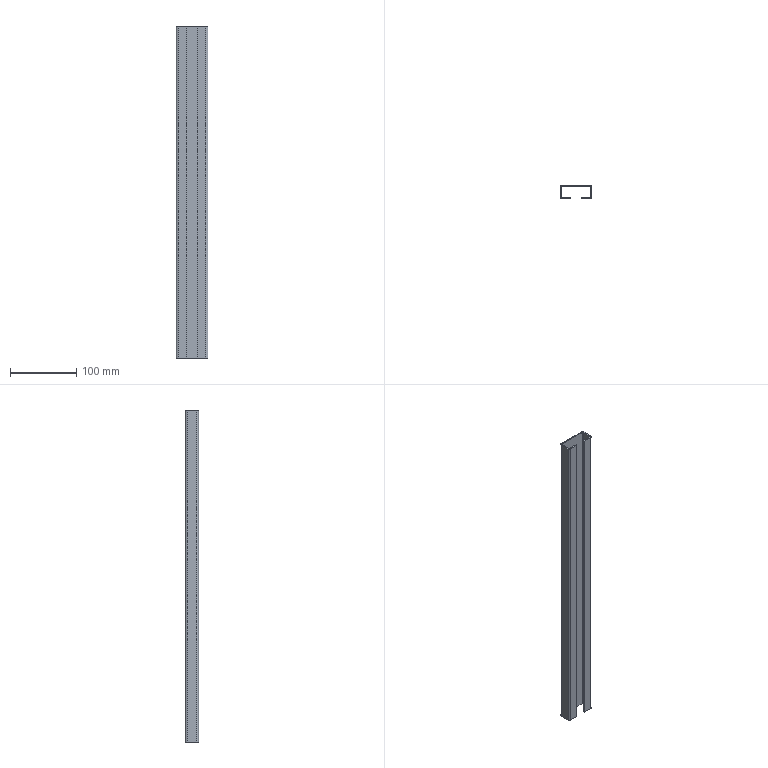Part | SolidWorks | features FlatPattern 1, SMBaseFlange 1, SheetMetal 1 | 1 solid | 38 faces | box 48 x 20 x 500 mm | volume 108566 mm3 | plane 30 | cylinder 8 | commonest cylinder face diameters 2 x4 6 x4
STEP:
#1=CARTESIAN_POINT('',(-24.,-17.,250.));
#2=VERTEX_POINT('',#1);
#3=CARTESIAN_POINT('',(-22.,-17.,250.));
#4=VERTEX_POINT('',#3);
#5=CARTESIAN_POINT('',(-24.,-17.,250.));
#6=DIRECTION('',(1.,0.,0.));
#7=VECTOR('',#6,1000.);
#8=LINE('',#5,#7);
#9=EDGE_CURVE('',#2,#4,#8,.T.);
#10=ORIENTED_EDGE('',*,*,#9,.F.);
#11=CARTESIAN_POINT('',(-21.,-20.,250.));
#12=VERTEX_POINT('',#11);
#13=CARTESIAN_POINT('',(-21.,-17.,250.));
#14=DIRECTION('',(0.,0.,-1.));
#15=DIRECTION('',(1.,0.,0.));
#16=AXIS2_PLACEMENT_3D('',#13,#14,#15);
#17=CIRCLE('',#16,3.);
#18=EDGE_CURVE('',#12,#2,#17,.T.);
#19=ORIENTED_EDGE('',*,*,#18,.F.);
#20=CARTESIAN_POINT('',(-21.,-18.,250.));
#21=VERTEX_POINT('',#20);
#22=CARTESIAN_POINT('',(-21.,-18.,250.));
#23=DIRECTION('',(0.,-1.,0.));
#24=VECTOR('',#23,1000.);
#25=LINE('',#22,#24);
#26=EDGE_CURVE('',#21,#12,#25,.T.);
#27=ORIENTED_EDGE('',*,*,#26,.F.);
#28=CARTESIAN_POINT('',(-21.,-17.,250.));
#29=DIRECTION('',(0.,0.,-1.));
#30=DIRECTION('',(1.,0.,0.));
#31=AXIS2_PLACEMENT_3D('',#28,#29,#30);
#32=CIRCLE('',#31,1.);
#33=EDGE_CURVE('',#21,#4,#32,.T.);
#34=ORIENTED_EDGE('',*,*,#33,.T.);
#35=EDGE_LOOP('',(#10,#19,#27,#34));
#36=FACE_OUTER_BOUND('',#35,.T.);
#37=CARTESIAN_POINT('',(-24.,-17.,250.));
#38=DIRECTION('',(0.,0.,1.));
#39=DIRECTION('',(1.,0.,0.));
#40=AXIS2_PLACEMENT_3D('',#37,#38,#39);
#41=PLANE('',#40);
#42=ADVANCED_FACE('',(#36),#41,.T.);
#43=CARTESIAN_POINT('',(-24.,-3.,250.));
#44=VERTEX_POINT('',#43);
#45=CARTESIAN_POINT('',(-24.,-20.,250.));
#46=DIRECTION('',(0.,1.,0.));
#47=VECTOR('',#46,1000.);
#48=LINE('',#45,#47);
#49=EDGE_CURVE('',#2,#44,#48,.T.);
#50=ORIENTED_EDGE('',*,*,#49,.F.);
#51=ORIENTED_EDGE('',*,*,#9,.T.);
#52=CARTESIAN_POINT('',(-22.,-3.,250.));
#53=VERTEX_POINT('',#52);
#54=CARTESIAN_POINT('',(-22.,-20.,250.));
#55=DIRECTION('',(0.,1.,0.));
#56=VECTOR('',#55,1000.);
#57=LINE('',#54,#56);
#58=EDGE_CURVE('',#4,#53,#57,.T.);
#59=ORIENTED_EDGE('',*,*,#58,.T.);
#60=CARTESIAN_POINT('',(-22.,-3.,250.));
#61=DIRECTION('',(-1.,0.,0.));
#62=VECTOR('',#61,1000.);
#63=LINE('',#60,#62);
#64=EDGE_CURVE('',#53,#44,#63,.T.);
#65=ORIENTED_EDGE('',*,*,#64,.T.);
#66=EDGE_LOOP('',(#50,#51,#59,#65));
#67=FACE_OUTER_BOUND('',#66,.T.);
#68=CARTESIAN_POINT('',(-21.,-18.,250.));
#69=DIRECTION('',(0.,0.,1.));
#70=DIRECTION('',(1.,0.,0.));
#71=AXIS2_PLACEMENT_3D('',#68,#69,#70);
#72=PLANE('',#71);
#73=ADVANCED_FACE('',(#67),#72,.T.);
#74=CARTESIAN_POINT('',(-21.,-20.,-250.));
#75=VERTEX_POINT('',#74);
#76=CARTESIAN_POINT('',(-21.,-18.,-250.));
#77=VERTEX_POINT('',#76);
#78=CARTESIAN_POINT('',(-21.,-20.,-250.));
#79=DIRECTION('',(0.,1.,0.));
#80=VECTOR('',#79,1000.);
#81=LINE('',#78,#80);
#82=EDGE_CURVE('',#75,#77,#81,.T.);
#83=ORIENTED_EDGE('',*,*,#82,.F.);
#84=CARTESIAN_POINT('',(-24.,-17.,-250.));
#85=VERTEX_POINT('',#84);
#86=CARTESIAN_POINT('',(-21.,-17.,-250.));
#87=DIRECTION('',(0.,0.,-1.));
#88=DIRECTION('',(1.,0.,0.));
#89=AXIS2_PLACEMENT_3D('',#86,#87,#88);
#90=CIRCLE('',#89,3.);
#91=EDGE_CURVE('',#75,#85,#90,.T.);
#92=ORIENTED_EDGE('',*,*,#91,.T.);
#93=CARTESIAN_POINT('',(-22.,-17.,-250.));
#94=VERTEX_POINT('',#93);
#95=CARTESIAN_POINT('',(-22.,-17.,-250.));
#96=DIRECTION('',(-1.,0.,0.));
#97=VECTOR('',#96,1000.);
#98=LINE('',#95,#97);
#99=EDGE_CURVE('',#94,#85,#98,.T.);
#100=ORIENTED_EDGE('',*,*,#99,.F.);
#101=CARTESIAN_POINT('',(-21.,-17.,-250.));
#102=DIRECTION('',(0.,0.,-1.));
#103=DIRECTION('',(1.,0.,0.));
#104=AXIS2_PLACEMENT_3D('',#101,#102,#103);
#105=CIRCLE('',#104,1.);
#106=EDGE_CURVE('',#77,#94,#105,.T.);
#107=ORIENTED_EDGE('',*,*,#106,.F.);
#108=EDGE_LOOP('',(#83,#92,#100,#107));
#109=FACE_OUTER_BOUND('',#108,.T.);
#110=CARTESIAN_POINT('',(-21.,-20.,-250.));
#111=DIRECTION('',(0.,0.,-1.));
#112=DIRECTION('',(-1.,0.,0.));
#113=AXIS2_PLACEMENT_3D('',#110,#111,#112);
#114=PLANE('',#113);
#115=ADVANCED_FACE('',(#109),#114,.T.);
#116=CARTESIAN_POINT('',(-8.,-20.,-250.));
#117=VERTEX_POINT('',#116);
#118=CARTESIAN_POINT('',(-8.,-20.,-250.));
#119=DIRECTION('',(-1.,0.,0.));
#120=VECTOR('',#119,1000.);
#121=LINE('',#118,#120);
#122=EDGE_CURVE('',#117,#75,#121,.T.);
#123=ORIENTED_EDGE('',*,*,#122,.T.);
#124=ORIENTED_EDGE('',*,*,#82,.T.);
#125=CARTESIAN_POINT('',(-8.,-18.,-250.));
#126=VERTEX_POINT('',#125);
#127=CARTESIAN_POINT('',(-8.,-18.,-250.));
#128=DIRECTION('',(-1.,0.,0.));
#129=VECTOR('',#128,1000.);
#130=LINE('',#127,#129);
#131=EDGE_CURVE('',#126,#77,#130,.T.);
#132=ORIENTED_EDGE('',*,*,#131,.F.);
#133=CARTESIAN_POINT('',(-8.,-18.,-250.));
#134=DIRECTION('',(0.,-1.,0.));
#135=VECTOR('',#134,1000.);
#136=LINE('',#133,#135);
#137=EDGE_CURVE('',#126,#117,#136,.T.);
#138=ORIENTED_EDGE('',*,*,#137,.T.);
#139=EDGE_LOOP('',(#123,#124,#132,#138));
#140=FACE_OUTER_BOUND('',#139,.T.);
#141=CARTESIAN_POINT('',(-22.,-17.,-250.));
#142=DIRECTION('',(0.,0.,-1.));
#143=DIRECTION('',(-1.,0.,0.));
#144=AXIS2_PLACEMENT_3D('',#141,#142,#143);
#145=PLANE('',#144);
#146=ADVANCED_FACE('',(#140),#145,.T.);
#147=CARTESIAN_POINT('',(-21.,0.,250.));
#148=VERTEX_POINT('',#147);
#149=CARTESIAN_POINT('',(-21.,-2.,250.));
#150=VERTEX_POINT('',#149);
#151=CARTESIAN_POINT('',(-21.,0.,250.));
#152=DIRECTION('',(0.,-1.,0.));
#153=VECTOR('',#152,1000.);
#154=LINE('',#151,#153);
#155=EDGE_CURVE('',#148,#150,#154,.T.);
#156=ORIENTED_EDGE('',*,*,#155,.F.);
#157=CARTESIAN_POINT('',(-21.,-3.,250.));
#158=DIRECTION('',(0.,0.,-1.));
#159=DIRECTION('',(1.,0.,0.));
#160=AXIS2_PLACEMENT_3D('',#157,#158,#159);
#161=CIRCLE('',#160,3.);
#162=EDGE_CURVE('',#44,#148,#161,.T.);
#163=ORIENTED_EDGE('',*,*,#162,.F.);
#164=ORIENTED_EDGE('',*,*,#64,.F.);
#165=CARTESIAN_POINT('',(-21.,-3.,250.));
#166=DIRECTION('',(0.,0.,-1.));
#167=DIRECTION('',(1.,0.,0.));
#168=AXIS2_PLACEMENT_3D('',#165,#166,#167);
#169=CIRCLE('',#168,1.);
#170=EDGE_CURVE('',#53,#150,#169,.T.);
#171=ORIENTED_EDGE('',*,*,#170,.T.);
#172=EDGE_LOOP('',(#156,#163,#164,#171));
#173=FACE_OUTER_BOUND('',#172,.T.);
#174=CARTESIAN_POINT('',(-21.,0.,250.));
#175=DIRECTION('',(0.,0.,1.));
#176=DIRECTION('',(1.,0.,0.));
#177=AXIS2_PLACEMENT_3D('',#174,#175,#176);
#178=PLANE('',#177);
#179=ADVANCED_FACE('',(#173),#178,.T.);
#180=CARTESIAN_POINT('',(21.,0.,250.));
#181=VERTEX_POINT('',#180);
#182=CARTESIAN_POINT('',(-24.,0.,250.));
#183=DIRECTION('',(1.,0.,0.));
#184=VECTOR('',#183,1000.);
#185=LINE('',#182,#184);
#186=EDGE_CURVE('',#148,#181,#185,.T.);
#187=ORIENTED_EDGE('',*,*,#186,.F.);
#188=ORIENTED_EDGE('',*,*,#155,.T.);
#189=CARTESIAN_POINT('',(21.,-2.,250.));
#190=VERTEX_POINT('',#189);
#191=CARTESIAN_POINT('',(-24.,-2.,250.));
#192=DIRECTION('',(1.,0.,0.));
#193=VECTOR('',#192,1000.);
#194=LINE('',#191,#193);
#195=EDGE_CURVE('',#150,#190,#194,.T.);
#196=ORIENTED_EDGE('',*,*,#195,.T.);
#197=CARTESIAN_POINT('',(21.,-2.,250.));
#198=DIRECTION('',(0.,1.,0.));
#199=VECTOR('',#198,1000.);
#200=LINE('',#197,#199);
#201=EDGE_CURVE('',#190,#181,#200,.T.);
#202=ORIENTED_EDGE('',*,*,#201,.T.);
#203=EDGE_LOOP('',(#187,#188,#196,#202));
#204=FACE_OUTER_BOUND('',#203,.T.);
#205=CARTESIAN_POINT('',(-22.,-3.,250.));
#206=DIRECTION('',(0.,0.,1.));
#207=DIRECTION('',(1.,0.,0.));
#208=AXIS2_PLACEMENT_3D('',#205,#206,#207);
#209=PLANE('',#208);
#210=ADVANCED_FACE('',(#204),#209,.T.);
#211=CARTESIAN_POINT('',(-24.,-3.,-250.));
#212=VERTEX_POINT('',#211);
#213=CARTESIAN_POINT('',(-22.,-3.,-250.));
#214=VERTEX_POINT('',#213);
#215=CARTESIAN_POINT('',(-24.,-3.,-250.));
#216=DIRECTION('',(1.,0.,0.));
#217=VECTOR('',#216,1000.);
#218=LINE('',#215,#217);
#219=EDGE_CURVE('',#212,#214,#218,.T.);
#220=ORIENTED_EDGE('',*,*,#219,.F.);
#221=CARTESIAN_POINT('',(-21.,0.,-250.));
#222=VERTEX_POINT('',#221);
#223=CARTESIAN_POINT('',(-21.,-3.,-250.));
#224=DIRECTION('',(0.,0.,-1.));
#225=DIRECTION('',(1.,0.,0.));
#226=AXIS2_PLACEMENT_3D('',#223,#224,#225);
#227=CIRCLE('',#226,3.);
#228=EDGE_CURVE('',#212,#222,#227,.T.);
#229=ORIENTED_EDGE('',*,*,#228,.T.);
#230=CARTESIAN_POINT('',(-21.,-2.,-250.));
#231=VERTEX_POINT('',#230);
#232=CARTESIAN_POINT('',(-21.,-2.,-250.));
#233=DIRECTION('',(0.,1.,0.));
#234=VECTOR('',#233,1000.);
#235=LINE('',#232,#234);
#236=EDGE_CURVE('',#231,#222,#235,.T.);
#237=ORIENTED_EDGE('',*,*,#236,.F.);
#238=CARTESIAN_POINT('',(-21.,-3.,-250.));
#239=DIRECTION('',(0.,0.,-1.));
#240=DIRECTION('',(1.,0.,0.));
#241=AXIS2_PLACEMENT_3D('',#238,#239,#240);
#242=CIRCLE('',#241,1.);
#243=EDGE_CURVE('',#214,#231,#242,.T.);
#244=ORIENTED_EDGE('',*,*,#243,.F.);
#245=EDGE_LOOP('',(#220,#229,#237,#244));
#246=FACE_OUTER_BOUND('',#245,.T.);
#247=CARTESIAN_POINT('',(-24.,-3.,-250.));
#248=DIRECTION('',(0.,0.,-1.));
#249=DIRECTION('',(-1.,0.,0.));
#250=AXIS2_PLACEMENT_3D('',#247,#248,#249);
#251=PLANE('',#250);
#252=ADVANCED_FACE('',(#246),#251,.T.);
#253=CARTESIAN_POINT('',(-24.,-20.,-250.));
#254=DIRECTION('',(0.,1.,0.));
#255=VECTOR('',#254,1000.);
#256=LINE('',#253,#255);
#257=EDGE_CURVE('',#85,#212,#256,.T.);
#258=ORIENTED_EDGE('',*,*,#257,.T.);
#259=ORIENTED_EDGE('',*,*,#219,.T.);
#260=CARTESIAN_POINT('',(-22.,-20.,-250.));
#261=DIRECTION('',(0.,1.,0.));
#262=VECTOR('',#261,1000.);
#263=LINE('',#260,#262);
#264=EDGE_CURVE('',#94,#214,#263,.T.);
#265=ORIENTED_EDGE('',*,*,#264,.F.);
#266=ORIENTED_EDGE('',*,*,#99,.T.);
#267=EDGE_LOOP('',(#258,#259,#265,#266));
#268=FACE_OUTER_BOUND('',#267,.T.);
#269=CARTESIAN_POINT('',(-21.,-2.,-250.));
#270=DIRECTION('',(0.,0.,-1.));
#271=DIRECTION('',(-1.,0.,0.));
#272=AXIS2_PLACEMENT_3D('',#269,#270,#271);
#273=PLANE('',#272);
#274=ADVANCED_FACE('',(#268),#273,.T.);
#275=CARTESIAN_POINT('',(24.,-3.,250.));
#276=VERTEX_POINT('',#275);
#277=CARTESIAN_POINT('',(22.,-3.,250.));
#278=VERTEX_POINT('',#277);
#279=CARTESIAN_POINT('',(24.,-3.,250.));
#280=DIRECTION('',(-1.,0.,0.));
#281=VECTOR('',#280,1000.);
#282=LINE('',#279,#281);
#283=EDGE_CURVE('',#276,#278,#282,.T.);
#284=ORIENTED_EDGE('',*,*,#283,.F.);
#285=CARTESIAN_POINT('',(21.,-3.,250.));
#286=DIRECTION('',(0.,0.,-1.));
#287=DIRECTION('',(1.,0.,0.));
#288=AXIS2_PLACEMENT_3D('',#285,#286,#287);
#289=CIRCLE('',#288,3.);
#290=EDGE_CURVE('',#181,#276,#289,.T.);
#291=ORIENTED_EDGE('',*,*,#290,.F.);
#292=ORIENTED_EDGE('',*,*,#201,.F.);
#293=CARTESIAN_POINT('',(21.,-3.,250.));
#294=DIRECTION('',(0.,0.,-1.));
#295=DIRECTION('',(1.,0.,0.));
#296=AXIS2_PLACEMENT_3D('',#293,#294,#295);
#297=CIRCLE('',#296,1.);
#298=EDGE_CURVE('',#190,#278,#297,.T.);
#299=ORIENTED_EDGE('',*,*,#298,.T.);
#300=EDGE_LOOP('',(#284,#291,#292,#299));
#301=FACE_OUTER_BOUND('',#300,.T.);
#302=CARTESIAN_POINT('',(24.,-3.,250.));
#303=DIRECTION('',(0.,0.,1.));
#304=DIRECTION('',(1.,0.,0.));
#305=AXIS2_PLACEMENT_3D('',#302,#303,#304);
#306=PLANE('',#305);
#307=ADVANCED_FACE('',(#301),#306,.T.);
#308=CARTESIAN_POINT('',(24.,-17.,250.));
#309=VERTEX_POINT('',#308);
#310=CARTESIAN_POINT('',(24.,0.,250.));
#311=DIRECTION('',(0.,-1.,0.));
#312=VECTOR('',#311,1000.);
#313=LINE('',#310,#312);
#314=EDGE_CURVE('',#276,#309,#313,.T.);
#315=ORIENTED_EDGE('',*,*,#314,.F.);
#316=ORIENTED_EDGE('',*,*,#283,.T.);
#317=CARTESIAN_POINT('',(22.,-17.,250.));
#318=VERTEX_POINT('',#317);
#319=CARTESIAN_POINT('',(22.,0.,250.));
#320=DIRECTION('',(0.,-1.,0.));
#321=VECTOR('',#320,1000.);
#322=LINE('',#319,#321);
#323=EDGE_CURVE('',#278,#318,#322,.T.);
#324=ORIENTED_EDGE('',*,*,#323,.T.);
#325=CARTESIAN_POINT('',(22.,-17.,250.));
#326=DIRECTION('',(1.,0.,0.));
#327=VECTOR('',#326,1000.);
#328=LINE('',#325,#327);
#329=EDGE_CURVE('',#318,#309,#328,.T.);
#330=ORIENTED_EDGE('',*,*,#329,.T.);
#331=EDGE_LOOP('',(#315,#316,#324,#330));
#332=FACE_OUTER_BOUND('',#331,.T.);
#333=CARTESIAN_POINT('',(21.,-2.,250.));
#334=DIRECTION('',(0.,0.,1.));
#335=DIRECTION('',(1.,0.,0.));
#336=AXIS2_PLACEMENT_3D('',#333,#334,#335);
#337=PLANE('',#336);
#338=ADVANCED_FACE('',(#332),#337,.T.);
#339=CARTESIAN_POINT('',(21.,0.,-250.));
#340=VERTEX_POINT('',#339);
#341=CARTESIAN_POINT('',(21.,-2.,-250.));
#342=VERTEX_POINT('',#341);
#343=CARTESIAN_POINT('',(21.,0.,-250.));
#344=DIRECTION('',(0.,-1.,0.));
#345=VECTOR('',#344,1000.);
#346=LINE('',#343,#345);
#347=EDGE_CURVE('',#340,#342,#346,.T.);
#348=ORIENTED_EDGE('',*,*,#347,.F.);
#349=CARTESIAN_POINT('',(24.,-3.,-250.));
#350=VERTEX_POINT('',#349);
#351=CARTESIAN_POINT('',(21.,-3.,-250.));
#352=DIRECTION('',(0.,0.,-1.));
#353=DIRECTION('',(1.,0.,0.));
#354=AXIS2_PLACEMENT_3D('',#351,#352,#353);
#355=CIRCLE('',#354,3.);
#356=EDGE_CURVE('',#340,#350,#355,.T.);
#357=ORIENTED_EDGE('',*,*,#356,.T.);
#358=CARTESIAN_POINT('',(22.,-3.,-250.));
#359=VERTEX_POINT('',#358);
#360=CARTESIAN_POINT('',(22.,-3.,-250.));
#361=DIRECTION('',(1.,0.,0.));
#362=VECTOR('',#361,1000.);
#363=LINE('',#360,#362);
#364=EDGE_CURVE('',#359,#350,#363,.T.);
#365=ORIENTED_EDGE('',*,*,#364,.F.);
#366=CARTESIAN_POINT('',(21.,-3.,-250.));
#367=DIRECTION('',(0.,0.,-1.));
#368=DIRECTION('',(1.,0.,0.));
#369=AXIS2_PLACEMENT_3D('',#366,#367,#368);
#370=CIRCLE('',#369,1.);
#371=EDGE_CURVE('',#342,#359,#370,.T.);
#372=ORIENTED_EDGE('',*,*,#371,.F.);
#373=EDGE_LOOP('',(#348,#357,#365,#372));
#374=FACE_OUTER_BOUND('',#373,.T.);
#375=CARTESIAN_POINT('',(21.,0.,-250.));
#376=DIRECTION('',(0.,0.,-1.));
#377=DIRECTION('',(-1.,0.,0.));
#378=AXIS2_PLACEMENT_3D('',#375,#376,#377);
#379=PLANE('',#378);
#380=ADVANCED_FACE('',(#374),#379,.T.);
#381=CARTESIAN_POINT('',(-24.,0.,-250.));
#382=DIRECTION('',(1.,0.,0.));
#383=VECTOR('',#382,1000.);
#384=LINE('',#381,#383);
#385=EDGE_CURVE('',#222,#340,#384,.T.);
#386=ORIENTED_EDGE('',*,*,#385,.T.);
#387=ORIENTED_EDGE('',*,*,#347,.T.);
#388=CARTESIAN_POINT('',(-24.,-2.,-250.));
#389=DIRECTION('',(1.,0.,0.));
#390=VECTOR('',#389,1000.);
#391=LINE('',#388,#390);
#392=EDGE_CURVE('',#231,#342,#391,.T.);
#393=ORIENTED_EDGE('',*,*,#392,.F.);
#394=ORIENTED_EDGE('',*,*,#236,.T.);
#395=EDGE_LOOP('',(#386,#387,#393,#394));
#396=FACE_OUTER_BOUND('',#395,.T.);
#397=CARTESIAN_POINT('',(22.,-3.,-250.));
#398=DIRECTION('',(0.,0.,-1.));
#399=DIRECTION('',(-1.,0.,0.));
#400=AXIS2_PLACEMENT_3D('',#397,#398,#399);
#401=PLANE('',#400);
#402=ADVANCED_FACE('',(#396),#401,.T.);
#403=CARTESIAN_POINT('',(21.,-20.,250.));
#404=VERTEX_POINT('',#403);
#405=CARTESIAN_POINT('',(21.,-18.,250.));
#406=VERTEX_POINT('',#405);
#407=CARTESIAN_POINT('',(21.,-20.,250.));
#408=DIRECTION('',(0.,1.,0.));
#409=VECTOR('',#408,1000.);
#410=LINE('',#407,#409);
#411=EDGE_CURVE('',#404,#406,#410,.T.);
#412=ORIENTED_EDGE('',*,*,#411,.F.);
#413=CARTESIAN_POINT('',(21.,-17.,250.));
#414=DIRECTION('',(0.,0.,-1.));
#415=DIRECTION('',(1.,0.,0.));
#416=AXIS2_PLACEMENT_3D('',#413,#414,#415);
#417=CIRCLE('',#416,3.);
#418=EDGE_CURVE('',#309,#404,#417,.T.);
#419=ORIENTED_EDGE('',*,*,#418,.F.);
#420=ORIENTED_EDGE('',*,*,#329,.F.);
#421=CARTESIAN_POINT('',(21.,-17.,250.));
#422=DIRECTION('',(0.,0.,-1.));
#423=DIRECTION('',(1.,0.,0.));
#424=AXIS2_PLACEMENT_3D('',#421,#422,#423);
#425=CIRCLE('',#424,1.);
#426=EDGE_CURVE('',#318,#406,#425,.T.);
#427=ORIENTED_EDGE('',*,*,#426,.T.);
#428=EDGE_LOOP('',(#412,#419,#420,#427));
#429=FACE_OUTER_BOUND('',#428,.T.);
#430=CARTESIAN_POINT('',(21.,-20.,250.));
#431=DIRECTION('',(0.,0.,1.));
#432=DIRECTION('',(1.,0.,0.));
#433=AXIS2_PLACEMENT_3D('',#430,#431,#432);
#434=PLANE('',#433);
#435=ADVANCED_FACE('',(#429),#434,.T.);
#436=CARTESIAN_POINT('',(8.,-20.,250.));
#437=VERTEX_POINT('',#436);
#438=CARTESIAN_POINT('',(24.,-20.,250.));
#439=DIRECTION('',(-1.,0.,0.));
#440=VECTOR('',#439,1000.);
#441=LINE('',#438,#440);
#442=EDGE_CURVE('',#404,#437,#441,.T.);
#443=ORIENTED_EDGE('',*,*,#442,.F.);
#444=ORIENTED_EDGE('',*,*,#411,.T.);
#445=CARTESIAN_POINT('',(8.,-18.,250.));
#446=VERTEX_POINT('',#445);
#447=CARTESIAN_POINT('',(24.,-18.,250.));
#448=DIRECTION('',(-1.,0.,0.));
#449=VECTOR('',#448,1000.);
#450=LINE('',#447,#449);
#451=EDGE_CURVE('',#406,#446,#450,.T.);
#452=ORIENTED_EDGE('',*,*,#451,.T.);
#453=CARTESIAN_POINT('',(8.,-20.,250.));
#454=DIRECTION('',(0.,1.,0.));
#455=VECTOR('',#454,1000.);
#456=LINE('',#453,#455);
#457=EDGE_CURVE('',#437,#446,#456,.T.);
#458=ORIENTED_EDGE('',*,*,#457,.F.);
#459=EDGE_LOOP('',(#443,#444,#452,#458));
#460=FACE_OUTER_BOUND('',#459,.T.);
#461=CARTESIAN_POINT('',(22.,-17.,250.));
#462=DIRECTION('',(0.,0.,1.));
#463=DIRECTION('',(1.,0.,0.));
#464=AXIS2_PLACEMENT_3D('',#461,#462,#463);
#465=PLANE('',#464);
#466=ADVANCED_FACE('',(#460),#465,.T.);
#467=CARTESIAN_POINT('',(24.,-17.,-250.));
#468=VERTEX_POINT('',#467);
#469=CARTESIAN_POINT('',(22.,-17.,-250.));
#470=VERTEX_POINT('',#469);
#471=CARTESIAN_POINT('',(24.,-17.,-250.));
#472=DIRECTION('',(-1.,0.,0.));
#473=VECTOR('',#472,1000.);
#474=LINE('',#471,#473);
#475=EDGE_CURVE('',#468,#470,#474,.T.);
#476=ORIENTED_EDGE('',*,*,#475,.F.);
#477=CARTESIAN_POINT('',(21.,-20.,-250.));
#478=VERTEX_POINT('',#477);
#479=CARTESIAN_POINT('',(21.,-17.,-250.));
#480=DIRECTION('',(0.,0.,-1.));
#481=DIRECTION('',(1.,0.,0.));
#482=AXIS2_PLACEMENT_3D('',#479,#480,#481);
#483=CIRCLE('',#482,3.);
#484=EDGE_CURVE('',#468,#478,#483,.T.);
#485=ORIENTED_EDGE('',*,*,#484,.T.);
#486=CARTESIAN_POINT('',(21.,-18.,-250.));
#487=VERTEX_POINT('',#486);
#488=CARTESIAN_POINT('',(21.,-18.,-250.));
#489=DIRECTION('',(0.,-1.,0.));
#490=VECTOR('',#489,1000.);
#491=LINE('',#488,#490);
#492=EDGE_CURVE('',#487,#478,#491,.T.);
#493=ORIENTED_EDGE('',*,*,#492,.F.);
#494=CARTESIAN_POINT('',(21.,-17.,-250.));
#495=DIRECTION('',(0.,0.,-1.));
#496=DIRECTION('',(1.,0.,0.));
#497=AXIS2_PLACEMENT_3D('',#494,#495,#496);
#498=CIRCLE('',#497,1.);
#499=EDGE_CURVE('',#470,#487,#498,.T.);
#500=ORIENTED_EDGE('',*,*,#499,.F.);
#501=EDGE_LOOP('',(#476,#485,#493,#500));
#502=FACE_OUTER_BOUND('',#501,.T.);
#503=CARTESIAN_POINT('',(24.,-17.,-250.));
#504=DIRECTION('',(0.,0.,-1.));
#505=DIRECTION('',(-1.,0.,0.));
#506=AXIS2_PLACEMENT_3D('',#503,#504,#505);
#507=PLANE('',#506);
#508=ADVANCED_FACE('',(#502),#507,.T.);
#509=CARTESIAN_POINT('',(24.,0.,-250.));
#510=DIRECTION('',(0.,-1.,0.));
#511=VECTOR('',#510,1000.);
#512=LINE('',#509,#511);
#513=EDGE_CURVE('',#350,#468,#512,.T.);
#514=ORIENTED_EDGE('',*,*,#513,.T.);
#515=ORIENTED_EDGE('',*,*,#475,.T.);
#516=CARTESIAN_POINT('',(22.,0.,-250.));
#517=DIRECTION('',(0.,-1.,0.));
#518=VECTOR('',#517,1000.);
#519=LINE('',#516,#518);
#520=EDGE_CURVE('',#359,#470,#519,.T.);
#521=ORIENTED_EDGE('',*,*,#520,.F.);
#522=ORIENTED_EDGE('',*,*,#364,.T.);
#523=EDGE_LOOP('',(#514,#515,#521,#522));
#524=FACE_OUTER_BOUND('',#523,.T.);
#525=CARTESIAN_POINT('',(21.,-18.,-250.));
#526=DIRECTION('',(0.,0.,-1.));
#527=DIRECTION('',(-1.,0.,0.));
#528=AXIS2_PLACEMENT_3D('',#525,#526,#527);
#529=PLANE('',#528);
#530=ADVANCED_FACE('',(#524),#529,.T.);
#531=CARTESIAN_POINT('',(8.,-18.,-250.));
#532=VERTEX_POINT('',#531);
#533=CARTESIAN_POINT('',(24.,-18.,-250.));
#534=DIRECTION('',(-1.,0.,0.));
#535=VECTOR('',#534,1000.);
#536=LINE('',#533,#535);
#537=EDGE_CURVE('',#487,#532,#536,.T.);
#538=ORIENTED_EDGE('',*,*,#537,.T.);
#539=CARTESIAN_POINT('',(8.,-18.,250.));
#540=DIRECTION('',(0.,0.,-1.));
#541=VECTOR('',#540,1000.);
#542=LINE('',#539,#541);
#543=EDGE_CURVE('',#446,#532,#542,.T.);
#544=ORIENTED_EDGE('',*,*,#543,.F.);
#545=ORIENTED_EDGE('',*,*,#451,.F.);
#546=CARTESIAN_POINT('',(21.,-18.,250.));
#547=DIRECTION('',(0.,0.,-1.));
#548=VECTOR('',#547,1000.);
#549=LINE('',#546,#548);
#550=EDGE_CURVE('',#406,#487,#549,.T.);
#551=ORIENTED_EDGE('',*,*,#550,.T.);
#552=EDGE_LOOP('',(#538,#544,#545,#551));
#553=FACE_OUTER_BOUND('',#552,.T.);
#554=CARTESIAN_POINT('',(24.,-18.,250.));
#555=DIRECTION('',(0.,-1.,0.));
#556=DIRECTION('',(1.,0.,0.));
#557=AXIS2_PLACEMENT_3D('',#554,#555,#556);
#558=PLANE('',#557);
#559=ADVANCED_FACE('',(#553),#558,.F.);
#560=CARTESIAN_POINT('',(8.,-20.,-250.));
#561=VERTEX_POINT('',#560);
#562=CARTESIAN_POINT('',(8.,-20.,-250.));
#563=DIRECTION('',(0.,1.,0.));
#564=VECTOR('',#563,1000.);
#565=LINE('',#562,#564);
#566=EDGE_CURVE('',#561,#532,#565,.T.);
#567=ORIENTED_EDGE('',*,*,#566,.F.);
#568=CARTESIAN_POINT('',(8.,-20.,250.));
#569=DIRECTION('',(0.,0.,-1.));
#570=VECTOR('',#569,1000.);
#571=LINE('',#568,#570);
#572=EDGE_CURVE('',#437,#561,#571,.T.);
#573=ORIENTED_EDGE('',*,*,#572,.F.);
#574=ORIENTED_EDGE('',*,*,#457,.T.);
#575=ORIENTED_EDGE('',*,*,#543,.T.);
#576=EDGE_LOOP('',(#567,#573,#574,#575));
#577=FACE_OUTER_BOUND('',#576,.T.);
#578=CARTESIAN_POINT('',(8.,-20.,250.));
#579=DIRECTION('',(-1.,0.,0.));
#580=DIRECTION('',(0.,0.,1.));
#581=AXIS2_PLACEMENT_3D('',#578,#579,#580);
#582=PLANE('',#581);
#583=ADVANCED_FACE('',(#577),#582,.T.);
#584=CARTESIAN_POINT('',(24.,-20.,-250.));
#585=DIRECTION('',(-1.,0.,0.));
#586=VECTOR('',#585,1000.);
#587=LINE('',#584,#586);
#588=EDGE_CURVE('',#478,#561,#587,.T.);
#589=ORIENTED_EDGE('',*,*,#588,.F.);
#590=CARTESIAN_POINT('',(21.,-20.,250.));
#591=DIRECTION('',(0.,0.,-1.));
#592=VECTOR('',#591,1000.);
#593=LINE('',#590,#592);
#594=EDGE_CURVE('',#404,#478,#593,.T.);
#595=ORIENTED_EDGE('',*,*,#594,.F.);
#596=ORIENTED_EDGE('',*,*,#442,.T.);
#597=ORIENTED_EDGE('',*,*,#572,.T.);
#598=EDGE_LOOP('',(#589,#595,#596,#597));
#599=FACE_OUTER_BOUND('',#598,.T.);
#600=CARTESIAN_POINT('',(24.,-20.,250.));
#601=DIRECTION('',(0.,-1.,0.));
#602=DIRECTION('',(1.,0.,0.));
#603=AXIS2_PLACEMENT_3D('',#600,#601,#602);
#604=PLANE('',#603);
#605=ADVANCED_FACE('',(#599),#604,.T.);
#606=ORIENTED_EDGE('',*,*,#484,.F.);
#607=CARTESIAN_POINT('',(24.,-17.,250.));
#608=DIRECTION('',(0.,0.,-1.));
#609=VECTOR('',#608,1000.);
#610=LINE('',#607,#609);
#611=EDGE_CURVE('',#309,#468,#610,.T.);
#612=ORIENTED_EDGE('',*,*,#611,.F.);
#613=ORIENTED_EDGE('',*,*,#418,.T.);
#614=ORIENTED_EDGE('',*,*,#594,.T.);
#615=EDGE_LOOP('',(#606,#612,#613,#614));
#616=FACE_OUTER_BOUND('',#615,.T.);
#617=CARTESIAN_POINT('',(21.,-17.,250.));
#618=DIRECTION('',(0.,0.,-1.));
#619=DIRECTION('',(-1.,0.,0.));
#620=AXIS2_PLACEMENT_3D('',#617,#618,#619);
#621=CYLINDRICAL_SURFACE('',#620,3.);
#622=ADVANCED_FACE('',(#616),#621,.T.);
#623=ORIENTED_EDGE('',*,*,#513,.F.);
#624=CARTESIAN_POINT('',(24.,-3.,250.));
#625=DIRECTION('',(0.,0.,-1.));
#626=VECTOR('',#625,1000.);
#627=LINE('',#624,#626);
#628=EDGE_CURVE('',#276,#350,#627,.T.);
#629=ORIENTED_EDGE('',*,*,#628,.F.);
#630=ORIENTED_EDGE('',*,*,#314,.T.);
#631=ORIENTED_EDGE('',*,*,#611,.T.);
#632=EDGE_LOOP('',(#623,#629,#630,#631));
#633=FACE_OUTER_BOUND('',#632,.T.);
#634=CARTESIAN_POINT('',(24.,0.,250.));
#635=DIRECTION('',(1.,0.,0.));
#636=DIRECTION('',(0.,0.,-1.));
#637=AXIS2_PLACEMENT_3D('',#634,#635,#636);
#638=PLANE('',#637);
#639=ADVANCED_FACE('',(#633),#638,.T.);
#640=ORIENTED_EDGE('',*,*,#356,.F.);
#641=CARTESIAN_POINT('',(21.,0.,250.));
#642=DIRECTION('',(0.,0.,-1.));
#643=VECTOR('',#642,1000.);
#644=LINE('',#641,#643);
#645=EDGE_CURVE('',#181,#340,#644,.T.);
#646=ORIENTED_EDGE('',*,*,#645,.F.);
#647=ORIENTED_EDGE('',*,*,#290,.T.);
#648=ORIENTED_EDGE('',*,*,#628,.T.);
#649=EDGE_LOOP('',(#640,#646,#647,#648));
#650=FACE_OUTER_BOUND('',#649,.T.);
#651=CARTESIAN_POINT('',(21.,-3.,250.));
#652=DIRECTION('',(0.,0.,-1.));
#653=DIRECTION('',(-1.,0.,0.));
#654=AXIS2_PLACEMENT_3D('',#651,#652,#653);
#655=CYLINDRICAL_SURFACE('',#654,3.);
#656=ADVANCED_FACE('',(#650),#655,.T.);
#657=ORIENTED_EDGE('',*,*,#385,.F.);
#658=CARTESIAN_POINT('',(-21.,0.,250.));
#659=DIRECTION('',(0.,0.,-1.));
#660=VECTOR('',#659,1000.);
#661=LINE('',#658,#660);
#662=EDGE_CURVE('',#148,#222,#661,.T.);
#663=ORIENTED_EDGE('',*,*,#662,.F.);
#664=ORIENTED_EDGE('',*,*,#186,.T.);
#665=ORIENTED_EDGE('',*,*,#645,.T.);
#666=EDGE_LOOP('',(#657,#663,#664,#665));
#667=FACE_OUTER_BOUND('',#666,.T.);
#668=CARTESIAN_POINT('',(-24.,0.,250.));
#669=DIRECTION('',(0.,1.,0.));
#670=DIRECTION('',(0.,0.,1.));
#671=AXIS2_PLACEMENT_3D('',#668,#669,#670);
#672=PLANE('',#671);
#673=ADVANCED_FACE('',(#667),#672,.T.);
#674=ORIENTED_EDGE('',*,*,#228,.F.);
#675=CARTESIAN_POINT('',(-24.,-3.,250.));
#676=DIRECTION('',(0.,0.,-1.));
#677=VECTOR('',#676,1000.);
#678=LINE('',#675,#677);
#679=EDGE_CURVE('',#44,#212,#678,.T.);
#680=ORIENTED_EDGE('',*,*,#679,.F.);
#681=ORIENTED_EDGE('',*,*,#162,.T.);
#682=ORIENTED_EDGE('',*,*,#662,.T.);
#683=EDGE_LOOP('',(#674,#680,#681,#682));
#684=FACE_OUTER_BOUND('',#683,.T.);
#685=CARTESIAN_POINT('',(-21.,-3.,250.));
#686=DIRECTION('',(0.,0.,-1.));
#687=DIRECTION('',(-1.,0.,0.));
#688=AXIS2_PLACEMENT_3D('',#685,#686,#687);
#689=CYLINDRICAL_SURFACE('',#688,3.);
#690=ADVANCED_FACE('',(#684),#689,.T.);
#691=ORIENTED_EDGE('',*,*,#257,.F.);
#692=CARTESIAN_POINT('',(-24.,-17.,250.));
#693=DIRECTION('',(0.,0.,-1.));
#694=VECTOR('',#693,1000.);
#695=LINE('',#692,#694);
#696=EDGE_CURVE('',#2,#85,#695,.T.);
#697=ORIENTED_EDGE('',*,*,#696,.F.);
#698=ORIENTED_EDGE('',*,*,#49,.T.);
#699=ORIENTED_EDGE('',*,*,#679,.T.);
#700=EDGE_LOOP('',(#691,#697,#698,#699));
#701=FACE_OUTER_BOUND('',#700,.T.);
#702=CARTESIAN_POINT('',(-24.,-20.,250.));
#703=DIRECTION('',(-1.,0.,0.));
#704=DIRECTION('',(0.,0.,1.));
#705=AXIS2_PLACEMENT_3D('',#702,#703,#704);
#706=PLANE('',#705);
#707=ADVANCED_FACE('',(#701),#706,.T.);
#708=ORIENTED_EDGE('',*,*,#91,.F.);
#709=CARTESIAN_POINT('',(-21.,-20.,250.));
#710=DIRECTION('',(0.,0.,-1.));
#711=VECTOR('',#710,1000.);
#712=LINE('',#709,#711);
#713=EDGE_CURVE('',#12,#75,#712,.T.);
#714=ORIENTED_EDGE('',*,*,#713,.F.);
#715=ORIENTED_EDGE('',*,*,#18,.T.);
#716=ORIENTED_EDGE('',*,*,#696,.T.);
#717=EDGE_LOOP('',(#708,#714,#715,#716));
#718=FACE_OUTER_BOUND('',#717,.T.);
#719=CARTESIAN_POINT('',(-21.,-17.,250.));
#720=DIRECTION('',(0.,0.,-1.));
#721=DIRECTION('',(-1.,0.,0.));
#722=AXIS2_PLACEMENT_3D('',#719,#720,#721);
#723=CYLINDRICAL_SURFACE('',#722,3.);
#724=ADVANCED_FACE('',(#718),#723,.T.);
#725=ORIENTED_EDGE('',*,*,#122,.F.);
#726=CARTESIAN_POINT('',(-8.,-20.,250.));
#727=VERTEX_POINT('',#726);
#728=CARTESIAN_POINT('',(-8.,-20.,250.));
#729=DIRECTION('',(0.,0.,-1.));
#730=VECTOR('',#729,1000.);
#731=LINE('',#728,#730);
#732=EDGE_CURVE('',#727,#117,#731,.T.);
#733=ORIENTED_EDGE('',*,*,#732,.F.);
#734=CARTESIAN_POINT('',(-8.,-20.,250.));
#735=DIRECTION('',(-1.,0.,0.));
#736=VECTOR('',#735,1000.);
#737=LINE('',#734,#736);
#738=EDGE_CURVE('',#727,#12,#737,.T.);
#739=ORIENTED_EDGE('',*,*,#738,.T.);
#740=ORIENTED_EDGE('',*,*,#713,.T.);
#741=EDGE_LOOP('',(#725,#733,#739,#740));
#742=FACE_OUTER_BOUND('',#741,.T.);
#743=CARTESIAN_POINT('',(-8.,-20.,250.));
#744=DIRECTION('',(0.,-1.,0.));
#745=DIRECTION('',(1.,0.,0.));
#746=AXIS2_PLACEMENT_3D('',#743,#744,#745);
#747=PLANE('',#746);
#748=ADVANCED_FACE('',(#742),#747,.T.);
#749=ORIENTED_EDGE('',*,*,#137,.F.);
#750=CARTESIAN_POINT('',(-8.,-18.,250.));
#751=VERTEX_POINT('',#750);
#752=CARTESIAN_POINT('',(-8.,-18.,250.));
#753=DIRECTION('',(0.,0.,-1.));
#754=VECTOR('',#753,1000.);
#755=LINE('',#752,#754);
#756=EDGE_CURVE('',#751,#126,#755,.T.);
#757=ORIENTED_EDGE('',*,*,#756,.F.);
#758=CARTESIAN_POINT('',(-8.,-18.,250.));
#759=DIRECTION('',(0.,-1.,0.));
#760=VECTOR('',#759,1000.);
#761=LINE('',#758,#760);
#762=EDGE_CURVE('',#751,#727,#761,.T.);
#763=ORIENTED_EDGE('',*,*,#762,.T.);
#764=ORIENTED_EDGE('',*,*,#732,.T.);
#765=EDGE_LOOP('',(#749,#757,#763,#764));
#766=FACE_OUTER_BOUND('',#765,.T.);
#767=CARTESIAN_POINT('',(-8.,-18.,250.));
#768=DIRECTION('',(1.,0.,0.));
#769=DIRECTION('',(0.,0.,-1.));
#770=AXIS2_PLACEMENT_3D('',#767,#768,#769);
#771=PLANE('',#770);
#772=ADVANCED_FACE('',(#766),#771,.T.);
#773=ORIENTED_EDGE('',*,*,#131,.T.);
#774=CARTESIAN_POINT('',(-21.,-18.,250.));
#775=DIRECTION('',(0.,0.,-1.));
#776=VECTOR('',#775,1000.);
#777=LINE('',#774,#776);
#778=EDGE_CURVE('',#21,#77,#777,.T.);
#779=ORIENTED_EDGE('',*,*,#778,.F.);
#780=CARTESIAN_POINT('',(-8.,-18.,250.));
#781=DIRECTION('',(-1.,0.,0.));
#782=VECTOR('',#781,1000.);
#783=LINE('',#780,#782);
#784=EDGE_CURVE('',#751,#21,#783,.T.);
#785=ORIENTED_EDGE('',*,*,#784,.F.);
#786=ORIENTED_EDGE('',*,*,#756,.T.);
#787=EDGE_LOOP('',(#773,#779,#785,#786));
#788=FACE_OUTER_BOUND('',#787,.T.);
#789=CARTESIAN_POINT('',(-8.,-18.,250.));
#790=DIRECTION('',(0.,-1.,0.));
#791=DIRECTION('',(1.,0.,0.));
#792=AXIS2_PLACEMENT_3D('',#789,#790,#791);
#793=PLANE('',#792);
#794=ADVANCED_FACE('',(#788),#793,.F.);
#795=ORIENTED_EDGE('',*,*,#106,.T.);
#796=CARTESIAN_POINT('',(-22.,-17.,250.));
#797=DIRECTION('',(0.,0.,-1.));
#798=VECTOR('',#797,1000.);
#799=LINE('',#796,#798);
#800=EDGE_CURVE('',#4,#94,#799,.T.);
#801=ORIENTED_EDGE('',*,*,#800,.F.);
#802=ORIENTED_EDGE('',*,*,#33,.F.);
#803=ORIENTED_EDGE('',*,*,#778,.T.);
#804=EDGE_LOOP('',(#795,#801,#802,#803));
#805=FACE_OUTER_BOUND('',#804,.T.);
#806=CARTESIAN_POINT('',(-21.,-17.,250.));
#807=DIRECTION('',(0.,0.,-1.));
#808=DIRECTION('',(-1.,0.,0.));
#809=AXIS2_PLACEMENT_3D('',#806,#807,#808);
#810=CYLINDRICAL_SURFACE('',#809,1.);
#811=ADVANCED_FACE('',(#805),#810,.F.);
#812=ORIENTED_EDGE('',*,*,#264,.T.);
#813=CARTESIAN_POINT('',(-22.,-3.,250.));
#814=DIRECTION('',(0.,0.,-1.));
#815=VECTOR('',#814,1000.);
#816=LINE('',#813,#815);
#817=EDGE_CURVE('',#53,#214,#816,.T.);
#818=ORIENTED_EDGE('',*,*,#817,.F.);
#819=ORIENTED_EDGE('',*,*,#58,.F.);
#820=ORIENTED_EDGE('',*,*,#800,.T.);
#821=EDGE_LOOP('',(#812,#818,#819,#820));
#822=FACE_OUTER_BOUND('',#821,.T.);
#823=CARTESIAN_POINT('',(-22.,-20.,250.));
#824=DIRECTION('',(-1.,0.,0.));
#825=DIRECTION('',(0.,0.,1.));
#826=AXIS2_PLACEMENT_3D('',#823,#824,#825);
#827=PLANE('',#826);
#828=ADVANCED_FACE('',(#822),#827,.F.);
#829=ORIENTED_EDGE('',*,*,#243,.T.);
#830=CARTESIAN_POINT('',(-21.,-2.,250.));
#831=DIRECTION('',(0.,0.,-1.));
#832=VECTOR('',#831,1000.);
#833=LINE('',#830,#832);
#834=EDGE_CURVE('',#150,#231,#833,.T.);
#835=ORIENTED_EDGE('',*,*,#834,.F.);
#836=ORIENTED_EDGE('',*,*,#170,.F.);
#837=ORIENTED_EDGE('',*,*,#817,.T.);
#838=EDGE_LOOP('',(#829,#835,#836,#837));
#839=FACE_OUTER_BOUND('',#838,.T.);
#840=CARTESIAN_POINT('',(-21.,-3.,250.));
#841=DIRECTION('',(0.,0.,-1.));
#842=DIRECTION('',(-1.,0.,0.));
#843=AXIS2_PLACEMENT_3D('',#840,#841,#842);
#844=CYLINDRICAL_SURFACE('',#843,1.);
#845=ADVANCED_FACE('',(#839),#844,.F.);
#846=ORIENTED_EDGE('',*,*,#392,.T.);
#847=CARTESIAN_POINT('',(21.,-2.,250.));
#848=DIRECTION('',(0.,0.,-1.));
#849=VECTOR('',#848,1000.);
#850=LINE('',#847,#849);
#851=EDGE_CURVE('',#190,#342,#850,.T.);
#852=ORIENTED_EDGE('',*,*,#851,.F.);
#853=ORIENTED_EDGE('',*,*,#195,.F.);
#854=ORIENTED_EDGE('',*,*,#834,.T.);
#855=EDGE_LOOP('',(#846,#852,#853,#854));
#856=FACE_OUTER_BOUND('',#855,.T.);
#857=CARTESIAN_POINT('',(-24.,-2.,250.));
#858=DIRECTION('',(0.,1.,0.));
#859=DIRECTION('',(0.,0.,1.));
#860=AXIS2_PLACEMENT_3D('',#857,#858,#859);
#861=PLANE('',#860);
#862=ADVANCED_FACE('',(#856),#861,.F.);
#863=ORIENTED_EDGE('',*,*,#371,.T.);
#864=CARTESIAN_POINT('',(22.,-3.,250.));
#865=DIRECTION('',(0.,0.,-1.));
#866=VECTOR('',#865,1000.);
#867=LINE('',#864,#866);
#868=EDGE_CURVE('',#278,#359,#867,.T.);
#869=ORIENTED_EDGE('',*,*,#868,.F.);
#870=ORIENTED_EDGE('',*,*,#298,.F.);
#871=ORIENTED_EDGE('',*,*,#851,.T.);
#872=EDGE_LOOP('',(#863,#869,#870,#871));
#873=FACE_OUTER_BOUND('',#872,.T.);
#874=CARTESIAN_POINT('',(21.,-3.,250.));
#875=DIRECTION('',(0.,0.,-1.));
#876=DIRECTION('',(-1.,0.,0.));
#877=AXIS2_PLACEMENT_3D('',#874,#875,#876);
#878=CYLINDRICAL_SURFACE('',#877,1.);
#879=ADVANCED_FACE('',(#873),#878,.F.);
#880=ORIENTED_EDGE('',*,*,#520,.T.);
#881=CARTESIAN_POINT('',(22.,-17.,250.));
#882=DIRECTION('',(0.,0.,-1.));
#883=VECTOR('',#882,1000.);
#884=LINE('',#881,#883);
#885=EDGE_CURVE('',#318,#470,#884,.T.);
#886=ORIENTED_EDGE('',*,*,#885,.F.);
#887=ORIENTED_EDGE('',*,*,#323,.F.);
#888=ORIENTED_EDGE('',*,*,#868,.T.);
#889=EDGE_LOOP('',(#880,#886,#887,#888));
#890=FACE_OUTER_BOUND('',#889,.T.);
#891=CARTESIAN_POINT('',(22.,0.,250.));
#892=DIRECTION('',(1.,0.,0.));
#893=DIRECTION('',(0.,0.,-1.));
#894=AXIS2_PLACEMENT_3D('',#891,#892,#893);
#895=PLANE('',#894);
#896=ADVANCED_FACE('',(#890),#895,.F.);
#897=ORIENTED_EDGE('',*,*,#499,.T.);
#898=ORIENTED_EDGE('',*,*,#550,.F.);
#899=ORIENTED_EDGE('',*,*,#426,.F.);
#900=ORIENTED_EDGE('',*,*,#885,.T.);
#901=EDGE_LOOP('',(#897,#898,#899,#900));
#902=FACE_OUTER_BOUND('',#901,.T.);
#903=CARTESIAN_POINT('',(21.,-17.,250.));
#904=DIRECTION('',(0.,0.,-1.));
#905=DIRECTION('',(-1.,0.,0.));
#906=AXIS2_PLACEMENT_3D('',#903,#904,#905);
#907=CYLINDRICAL_SURFACE('',#906,1.);
#908=ADVANCED_FACE('',(#902),#907,.F.);
#909=ORIENTED_EDGE('',*,*,#784,.T.);
#910=ORIENTED_EDGE('',*,*,#26,.T.);
#911=ORIENTED_EDGE('',*,*,#738,.F.);
#912=ORIENTED_EDGE('',*,*,#762,.F.);
#913=EDGE_LOOP('',(#909,#910,#911,#912));
#914=FACE_OUTER_BOUND('',#913,.T.);
#915=CARTESIAN_POINT('',(21.,-17.,250.));
#916=DIRECTION('',(0.,0.,1.));
#917=DIRECTION('',(1.,0.,0.));
#918=AXIS2_PLACEMENT_3D('',#915,#916,#917);
#919=PLANE('',#918);
#920=ADVANCED_FACE('',(#914),#919,.T.);
#921=ORIENTED_EDGE('',*,*,#537,.F.);
#922=ORIENTED_EDGE('',*,*,#492,.T.);
#923=ORIENTED_EDGE('',*,*,#588,.T.);
#924=ORIENTED_EDGE('',*,*,#566,.T.);
#925=EDGE_LOOP('',(#921,#922,#923,#924));
#926=FACE_OUTER_BOUND('',#925,.T.);
#927=CARTESIAN_POINT('',(21.,-17.,-250.));
#928=DIRECTION('',(0.,0.,1.));
#929=DIRECTION('',(1.,0.,0.));
#930=AXIS2_PLACEMENT_3D('',#927,#928,#929);
#931=PLANE('',#930);
#932=ADVANCED_FACE('',(#926),#931,.F.);
#933=CLOSED_SHELL('',(#42,#73,#115,#146,#179,#210,#252,#274,#307,#338,#380,#402,#435,#466,#508,#530,#559,#583,#605,#622,#639,#656,#673,#690,#707,#724,#748,#772,#794,#811,#828,#845,#862,#879,#896,#908,#920,#932));
#934=MANIFOLD_SOLID_BREP('',#933);
#935=CARTESIAN_POINT('',(0.,0.,0.));
#936=DIRECTION('',(0.,0.,1.));
#937=DIRECTION('',(1.,0.,0.));
#938=AXIS2_PLACEMENT_3D('',#935,#936,#937);
#939=(LENGTH_UNIT()NAMED_UNIT(*)SI_UNIT(.MILLI.,.METRE.));
#940=UNCERTAINTY_MEASURE_WITH_UNIT(LENGTH_MEASURE(0.00001),#939,'','');
#941=(NAMED_UNIT(*)PLANE_ANGLE_UNIT()SI_UNIT($,.RADIAN.));
#942=(NAMED_UNIT(*)SI_UNIT($,.STERADIAN.)SOLID_ANGLE_UNIT());
#943=(GEOMETRIC_REPRESENTATION_CONTEXT(3)GLOBAL_UNCERTAINTY_ASSIGNED_CONTEXT((#940))GLOBAL_UNIT_ASSIGNED_CONTEXT((#939,#941,#942))REPRESENTATION_CONTEXT('',''));
#944=ADVANCED_BREP_SHAPE_REPRESENTATION('',(#934,#938),#943);